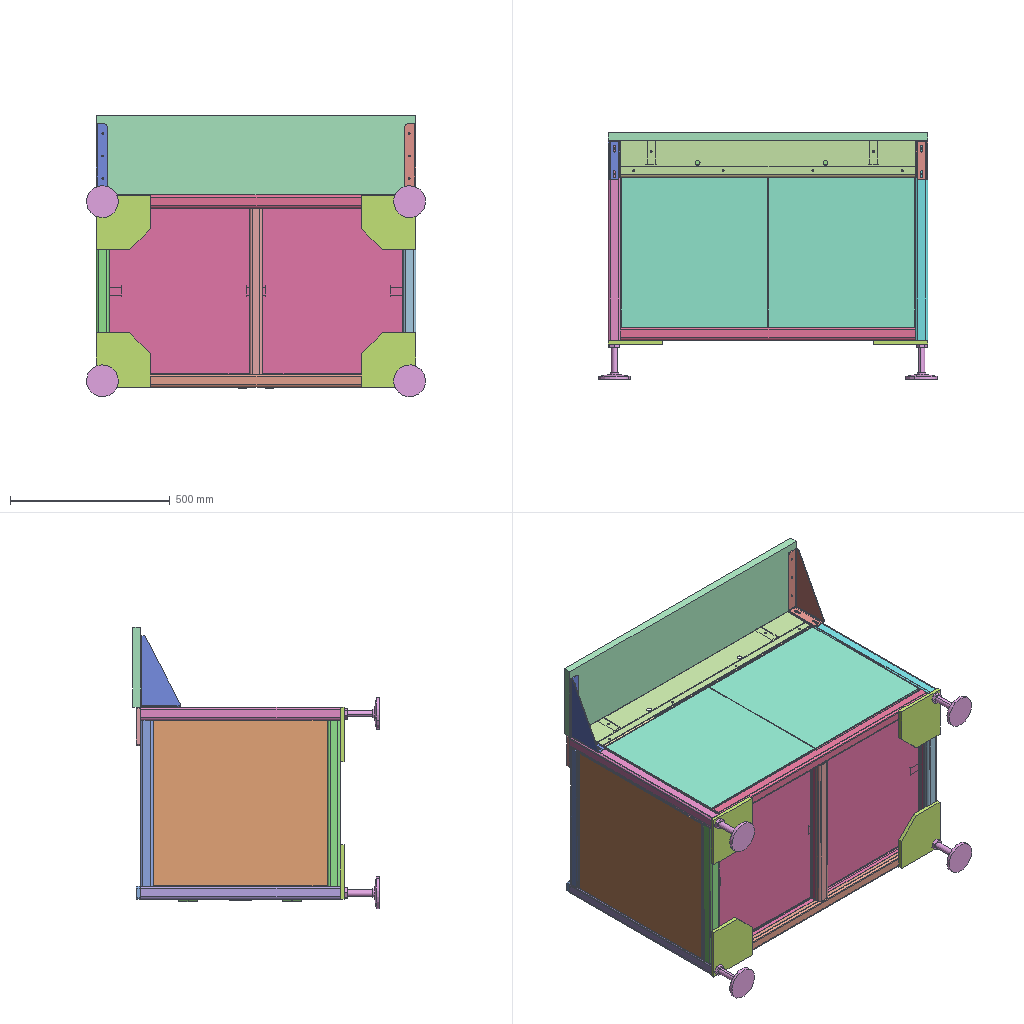Assembly | SolidWorks | 25 different items | 46 placed | box 1060 x 771 x 880 mm
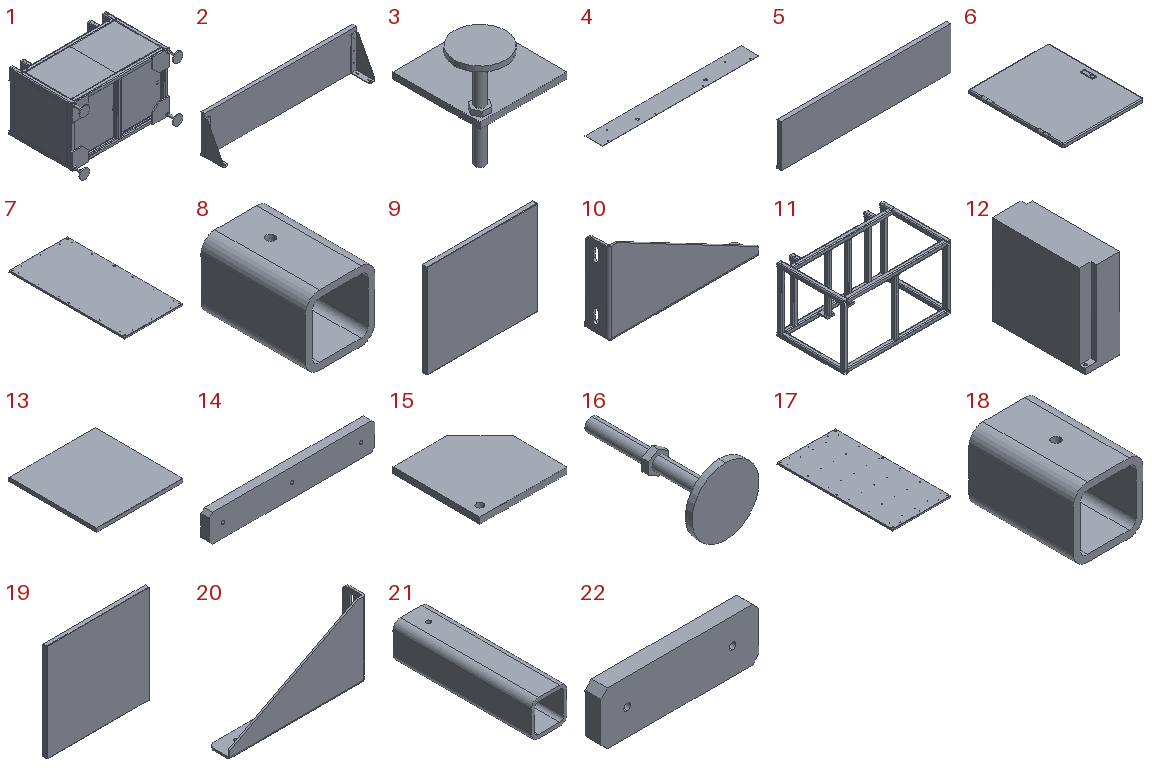Parts list (item | name | quantity | parent item | size | volume | features):
1 | (subassembly) | x1 | - | 1060 x 759 x 660 mm | 11116093 mm3 | features Cut 1
2 | (subassembly) | x1 | - | 1000 x 148 x 250 mm | 6407713 mm3 | features LocalLPattern 1, MateUpdatePoint 1, ReferencePattern 1
3 | (subassembly) | x4 | in 1 | 200 x 200 x 200 mm | 476868 mm3 | -
4 | - | x1 | - | 920 x 105 x 1 mm | 96077 mm3 | features Cut 1, Extrusion 1, HoleWzd 1
5 | - | x1 | in 2 | 1000 x 25 x 250 mm | 6250000 mm3 | features Fillet 3, Cut 1, Extrusion 1, LPattern 1
6 | - | x2 | in 1 | 467.5 x 545 x 27.5 mm | 335829 mm3 | features Cut 4, Boss 3, Extrusion 1, Fillet 1, LibraryFeature 1, MirrorPattern 1, Shell 1
7 | - | x1 | - | 460 x 910 x 12 mm | 667248 mm3 | features EdgeFlange 4, 3DProfileFeature 3, HoleWzd 3, MirrorPattern 3, FlatPattern 1, SMBaseFlange 1, SheetMetal 1
8 | - | x2 | in 1 | 40 x 60 x 40 mm | 31931 mm3 | features HoleWzd 1, WeldMemberFeat 1, WeldmentFeature 1
9 | - | x2 | in 1 | 520 x 21 x 440 mm | 266132 mm3 | features EdgeFlange 4, FlatPattern 1, SMBaseFlange 1, SheetMetal 1
10 | - | x1 | in 2 | 223 x 36 x 123 mm | 78856 mm3 | features Cut 1, EdgeFlange 1, Fillet 1, FlatPattern 1, HoleWzd 1, LPattern 1, SMBaseFlange 1, SheetMetal 1
11 | - | x1 | in 1 | 1000 x 625 x 600 mm | 6055462 mm3 | features DelFace 22, WeldCornerFeat 15, CombineBodies 7, WeldMemberFeat 6, 3DProfileFeature 2, Boss 2, DeleteBody 2, HoleWzd 2, MoveCopyBody 2, WeldmentFeature 1
12 | - | x2 | - | 60.2 x 162 x 155.9 mm | 1476236 mm3 | features Cut 2, Extrusion 1
13 | - | x2 | in 1 | 460 x 470 x 20 mm | 276608 mm3 | features Cut 4, Boss 3, Extrusion 1, Fillet 1, LibraryFeature 1, MirrorPattern 1, Shell 1
14 | - | x2 | in 1 | 240 x 12 x 40 mm | 113893 mm3 | features Chamfer 1, Extrusion 1, HoleWzd 1
15 | - | x4 | in 3 | 170 x 170 x 12 mm | 319603 mm3 | features HoleWzd 2, Chamfer 1, Extrusion 1
16 | - | x4 | in 3 | 100 x 200 x 100 mm | 157266 mm3 | features Boss 1, Revolution 1
17 | - | x1 | - | 460 x 910 x 12 mm | 667017 mm3 | features EdgeFlange 4, 3DProfileFeature 3, HoleWzd 3, MirrorPattern 2, FlatPattern 1, LPattern 1, SMBaseFlange 1, SheetMetal 1
18 | - | x2 | in 1 | 40 x 60 x 40 mm | 31931 mm3 | features HoleWzd 1, WeldMemberFeat 1, WeldmentFeature 1
19 | - | x2 | in 1 | 545 x 21 x 520 mm | 324842 mm3 | features EdgeFlange 4, Cut 1, FlatPattern 1, SMBaseFlange 1, SheetMetal 1
20 | - | x1 | in 2 | 223 x 36 x 123 mm | 78856 mm3 | features MirrorStock 1
21 | - | x2 | in 1 | 40 x 155 x 40 mm | 82736 mm3 | features HoleWzd 1, WeldMemberFeat 1, WeldmentFeature 1
22 | - | x4 | in 1 | 120 x 12 x 40 mm | 56529 mm3 | features Chamfer 1, Extrusion 1, HoleWzd 1
23 | FW6590F | x1 | - | - | - | -
24 | Button1 | x1 | - | - | - | -
25 | Connecting Block | x1 | - | - | - | -
Mates (type | each side: item.copy, entity, surface, feature):
In the top assembly
Coincident | 11.1 face plane Structural Member3 | 10.1 face plane Edge Flange1
DistanceDim | 22.1 face plane Extrude1 | 5.1 face plane Extrude1
Coincident | 11.1 face plane Structural Member1 | 10.1 face plane Base Flange1
Coincident | 11.1 face plane Structural Member3 | 4.1 face plane Extrude1
Coincident | 5.1 face plane Extrude1 | 4.1 face plane Extrude1
Coincident | 11.1 plane | 4.1 plane
Coincident | 8.1 face plane Structural Member1 | 7.1 face plane Edge Flange1
Concentric | 8.1 face cylinder M6 Tapped Hole1 | 7.1 face cylinder M6 Clearance Hole1
Concentric | 7.1 face cylinder M6 Clearance Hole1 | 17.1 face cylinder M6 Clearance Hole1 | 2 times
Coincident | 21.1 face plane Structural Member1 | 17.1 face plane Edge Flange1
Coincident | 7.1 face plane Base Flange1 | 12.1 face plane Extrude1
DistanceDim | 7.1 plane | 12.1 face plane Extrude1
DistanceDim | 7.1 face plane Edge Flange1 | 12.1 face plane Extrude1
Coincident | 7.1 face plane Base Flange1 | 12.2 face plane Extrude1
Coincident | 12.1 face plane Extrude1 | 12.2 face plane Extrude1
DistanceDim | 7.1 plane | 12.2 face plane Extrude1
Concentric | 21.2 face cylinder M6 Tapped Hole1 | 7.1 face cylinder M6 Clearance Hole1
In subassembly 2
Coincident | 5.2 face plane Extrude1 | 10.2 face plane Edge Flange1 | 2 times
Coincident | 5.2 face plane Extrude1 | 10.2 face plane Base Flange1
Coincident | 5.2 face plane Extrude1 | 20.1 face plane 11-02 Mirror | 3 times
In subassembly 1
Coincident | 11.2 face plane Structural Member2 | 22.2 face plane Extrude1 | 2 times
Coincident | 11.2 face plane Structural Member1 | 22.2 face plane Extrude1
Coincident | 11.2 face plane Structural Member2 | 22.3 face plane Extrude1
Coincident | 11.2 face plane Structural Member5 | 22.3 face plane Extrude1 | 2 times
Coincident | 11.2 face plane Structural Member6 | 22.4 face plane Extrude1
Coincident | 22.4 face plane Extrude1 | 22.5 face plane Extrude1
Coincident | 11.2 face plane Structural Member2 | 22.4 face plane Extrude1
Coincident | 11.2 face plane Structural Member1 | 22.4 face plane Extrude1
Coincident | 11.2 face plane Structural Member6 | 22.5 face plane Extrude1 | 2 times
Coincident | 11.2 face plane Structural Member2 | 22.6 face | 2 times
Coincident | 22.6 face | 22.7 face | 2 times
Coincident | 11.2 face plane Structural Member2 | 22.7 face
DistanceDim | 22.6 face | 11.2 face plane Extrude2
Coincident | 11.2 face plane Structural Member2 | 14.1 face plane Extrude1 | 2 times
Coincident | 11.2 face plane Structural Member1 | 14.1 face plane Extrude1
Coincident | 11.2 face plane Structural Member2 | 14.2 face plane Extrude1 | 2 times
Coincident | 11.2 face plane Structural Member1 | 14.2 face plane Extrude1
Coincident | 11.2 face plane Structural Member4 | 15.1 face plane Extrude1 | 3 times
Coincident | 11.2 face plane Structural Member4 | 15.2 face plane Extrude1 | 2 times
Coincident | 11.2 face plane Structural Member4 | 15.3 face plane Extrude1 | 3 times
Coincident | 11.2 face plane Structural Member4 | 15.4 face plane Extrude1 | 3 times
Coincident | 11.2 face plane Structural Member1 | 15.2 face plane Extrude1
Coincident | 11.2 face plane Structural Member2 | 22.8 face | 2 times
Coincident | 22.8 face | 22.9 face
Coincident | 11.2 face plane Structural Member3 | 22.8 face
Coincident | 11.2 face plane Structural Member2 | 22.9 face
Coincident | 11.2 face plane Structural Member3 | 22.9 face
Coincident | 11.2 face plane Structural Member3 | 13.1 face plane Extrude1
Coincident | 11.2 face plane Structural Member1 | 13.1 face plane Extrude1 | 2 times
Coincident | 11.2 face plane Structural Member1 | 13.2 face plane Extrude1
Coincident | 11.2 face plane Structural Member4 | 13.2 face plane Extrude1 | 2 times
Coincident | 11.2 face plane Structural Member1 | 19.1 face plane Base Flange1
Coincident | 11.2 face plane Structural Member1 | 19.1 face plane Edge Flange3
Coincident | 11.2 face plane Structural Member4 | 19.1 face plane Edge Flange2
Coincident | 11.2 face plane Structural Member4 | 19.2 face plane
Coincident | 11.2 face plane Structural Member1 | 6.1 face plane Extrude1 | 2 times
Coincident | 11.2 face plane Structural Member2 | 6.1 face plane Extrude1
Coincident | 11.2 face plane Structural Member1 | 6.2 face plane Extrude1
Coincident | 11.2 face plane Structural Member4 | 6.2 face plane Extrude1 | 2 times
Coincident | 11.2 face plane Structural Member4 | 9.1 face plane Base Flange1
Coincident | 11.2 face plane Structural Member4 | 9.1 face plane Edge Flange3
Coincident | 11.2 face plane Structural Member4 | 9.1 face plane Edge Flange2
Coincident | 9.1 face plane Base Flange1 | 9.2 face plane Base Flange1
Coincident | 11.2 face plane Structural Member4 | 9.2 face plane Edge Flange4
Coincident | 11.2 face plane Structural Member4 | 9.2 face plane Edge Flange1
Coincident | 11.2 face plane Structural Member2 | 22.10 face | 2 times
Coincident | 11.2 plane | 22.10 plane
Coincident | 11.2 face plane Structural Member4 | 8.2 face plane Structural Member1
DistanceDim | 11.2 face plane Structural Member4 | 8.2 face plane Structural Member1
Coincident | 11.2 plane | 8.2 plane
Coincident | 8.2 face plane Structural Member1 | 8.3 face plane Structural Member1
Coincident | 11.2 face plane Structural Member4 | 8.3 face plane Structural Member1
DistanceDim | 11.2 face plane Structural Member4 | 8.3 face plane Structural Member1
Coincident | 11.2 face plane Structural Member5 | 21.3 face plane Structural Member1
Coincident | 8.2 face plane Structural Member1 | 21.3 face plane Structural Member1
Coincident | 11.2 face plane Structural Member2 | 21.4 face plane Structural Member1 | 2 times
Coincident | 8.2 face plane Structural Member1 | 21.4 face plane Structural Member1
Coincident | 11.2 face plane Structural Member2 | 21.3 face plane Structural Member1
Coincident | 11.2 face plane Structural Member4 | 18.1 face plane Structural Member1
Coincident | 8.2 face plane Structural Member1 | 18.1 face plane Structural Member1
Coincident | 11.2 plane | 18.1 plane
Coincident | 11.2 face plane Structural Member2 | 18.2 face plane Structural Member1
Coincident | 21.4 face plane Structural Member1 | 18.2 face plane Structural Member1
Width | 18.2 face plane Structural Member1 | 18.2 face plane Structural Member1 | 11.2 face plane Structural Member2 | 11.2 face plane Structural Member2
In subassembly 3
Concentric | 15.5 face cylinder M16x2.0 Tapped Hole1 | 16.1 face cylinder Revolve1
Coincident | 15.5 face plane Extrude1 | 16.1 face plane Extrude1